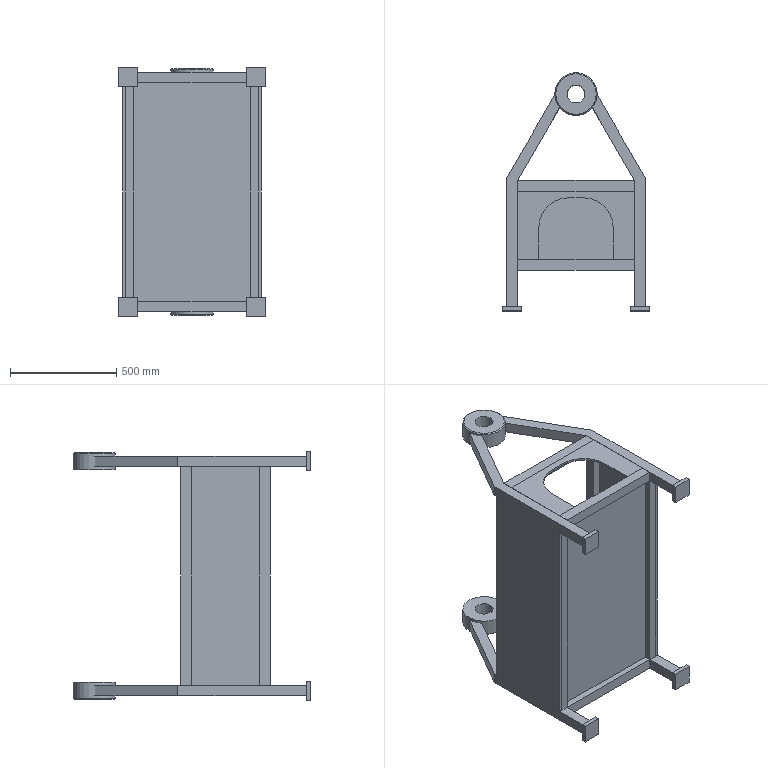Part | NX | features DATUM_CSYS 11, EXTRUDE 10, SKETCH 10, EXTRACT_BODY 8, Container 2, Geometry Instance 2, LINKED_FACE 2, CHAMFER 1, CYLINDER 1, LINKED_CURVE 1 | 23 solids | 150 faces | box 690 x 1120 x 1170 mm | volume 52680048 mm3 | plane 142 | cylinder 6 | cone 2 | commonest cylinder face diameters 84 x2 200 x2 280 x2